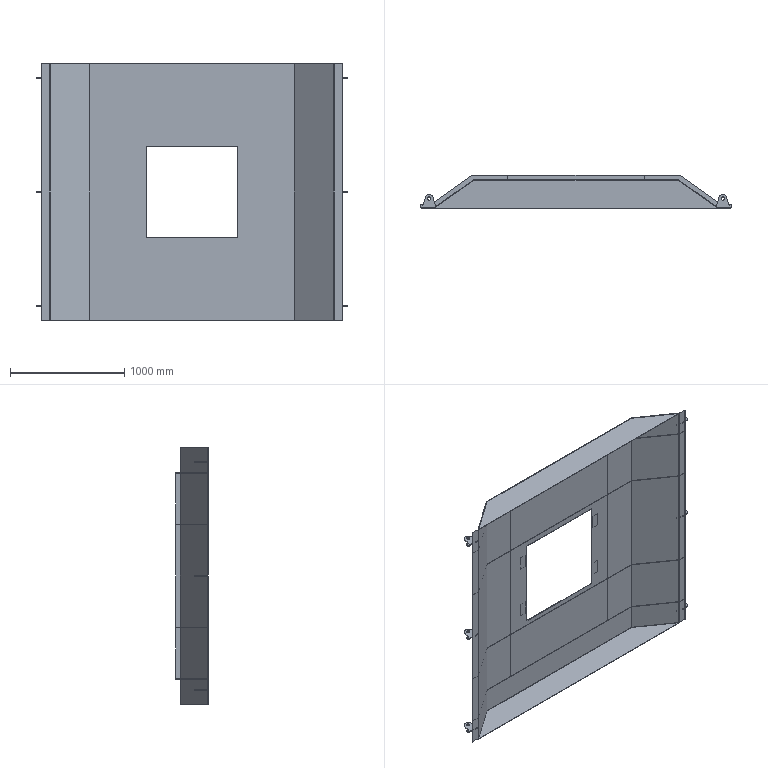Part | STEP file | Seal cover 1_Default<As machined> | 23 solids | 232 faces | box 2723 x 286.121 x 2250 mm | volume 29731618 mm3 | plane 194 | cylinder 38 | commonest cylinder face diameters 30 x18 16 x6 70 x6 6 x4 14 x4